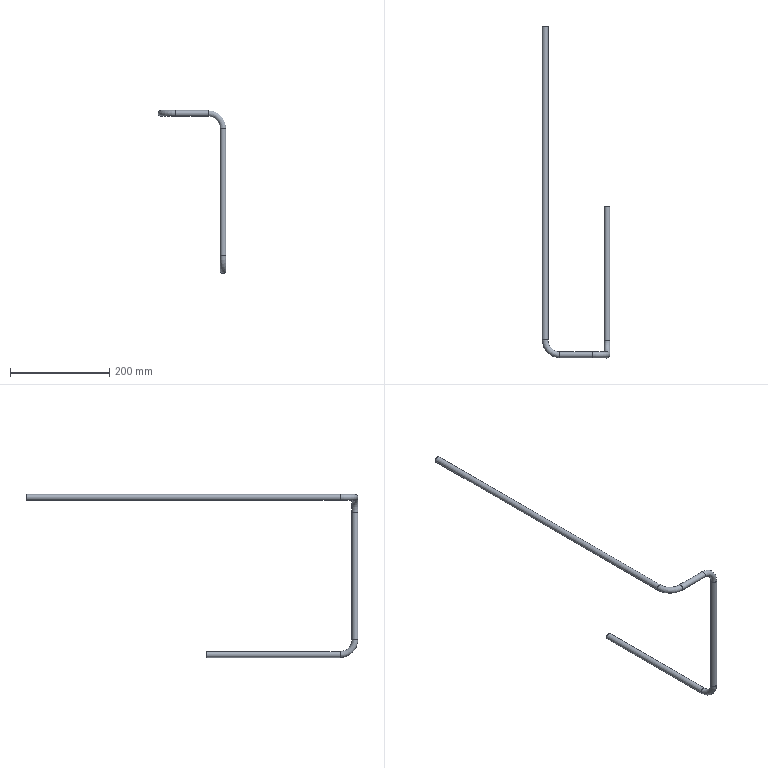Part | NX | features solid 2 | 1 solid | 9 faces | box 137 x 670 x 329.5 mm | volume 154703 mm3 | cylinder 4 | torus 3 | plane 2 | commonest cylinder face diameters 12 x4
STEP:
#1=CARTESIAN_POINT('',(125.,135.,-479.));
#2=VERTEX_POINT('',#1);
#3=CARTESIAN_POINT('',(125.,135.,-485.));
#4=DIRECTION('',(0.,1.,0.));
#5=DIRECTION('',(0.,0.,1.));
#6=AXIS2_PLACEMENT_3D('',#3,#4,#5);
#7=CIRCLE('',#6,6.);
#8=EDGE_CURVE('',#2,#2,#7,.T.);
#9=ORIENTED_EDGE('',*,*,#8,.T.);
#10=EDGE_LOOP('',(#9));
#11=FACE_BOUND('',#10,.T.);
#12=CARTESIAN_POINT('',(125.,405.,-479.));
#13=VERTEX_POINT('',#12);
#14=CARTESIAN_POINT('',(125.,405.,-485.));
#15=DIRECTION('',(0.,1.,0.));
#16=DIRECTION('',(0.,0.,1.));
#17=AXIS2_PLACEMENT_3D('',#14,#15,#16);
#18=CIRCLE('',#17,6.);
#19=EDGE_CURVE('',#13,#13,#18,.T.);
#20=ORIENTED_EDGE('',*,*,#19,.F.);
#21=EDGE_LOOP('',(#20));
#22=FACE_BOUND('',#21,.T.);
#23=CARTESIAN_POINT('',(125.,135.,-485.));
#24=DIRECTION('',(0.,1.,0.));
#25=DIRECTION('',(-1.,0.,0.));
#26=AXIS2_PLACEMENT_3D('',#23,#24,#25);
#27=CYLINDRICAL_SURFACE('',#26,6.);
#28=ADVANCED_FACE('',(#11,#22),#27,.T.);
#29=CARTESIAN_POINT('',(125.,111.,-455.));
#30=VERTEX_POINT('',#29);
#31=CARTESIAN_POINT('',(125.,105.,-455.));
#32=DIRECTION('',(0.,0.,-1.));
#33=DIRECTION('',(0.,1.,0.));
#34=AXIS2_PLACEMENT_3D('',#31,#32,#33);
#35=CIRCLE('',#34,6.);
#36=EDGE_CURVE('',#30,#30,#35,.T.);
#37=ORIENTED_EDGE('',*,*,#36,.T.);
#38=EDGE_LOOP('',(#37));
#39=FACE_BOUND('',#38,.T.);
#40=ORIENTED_EDGE('',*,*,#8,.F.);
#41=EDGE_LOOP('',(#40));
#42=FACE_BOUND('',#41,.T.);
#43=CARTESIAN_POINT('',(125.,135.,-455.));
#44=DIRECTION('',(1.,0.,0.));
#45=DIRECTION('',(0.,0.,-1.));
#46=AXIS2_PLACEMENT_3D('',#43,#44,#45);
#47=TOROIDAL_SURFACE('',#46,30.,6.);
#48=ADVANCED_FACE('',(#39,#42),#47,.T.);
#49=CARTESIAN_POINT('',(125.,111.,-197.5));
#50=VERTEX_POINT('',#49);
#51=CARTESIAN_POINT('',(125.,105.,-197.5));
#52=DIRECTION('',(0.,0.,-1.));
#53=DIRECTION('',(0.,1.,0.));
#54=AXIS2_PLACEMENT_3D('',#51,#52,#53);
#55=CIRCLE('',#54,6.);
#56=EDGE_CURVE('',#50,#50,#55,.T.);
#57=ORIENTED_EDGE('',*,*,#56,.T.);
#58=EDGE_LOOP('',(#57));
#59=FACE_BOUND('',#58,.T.);
#60=ORIENTED_EDGE('',*,*,#36,.F.);
#61=EDGE_LOOP('',(#60));
#62=FACE_BOUND('',#61,.T.);
#63=CARTESIAN_POINT('',(125.,105.,-197.5));
#64=DIRECTION('',(0.,0.,-1.));
#65=DIRECTION('',(-1.,0.,0.));
#66=AXIS2_PLACEMENT_3D('',#63,#64,#65);
#67=CYLINDRICAL_SURFACE('',#66,6.);
#68=ADVANCED_FACE('',(#59,#62),#67,.T.);
#69=CARTESIAN_POINT('',(95.,111.,-167.5));
#70=VERTEX_POINT('',#69);
#71=CARTESIAN_POINT('',(95.,105.,-167.5));
#72=DIRECTION('',(1.,0.,0.));
#73=DIRECTION('',(0.,1.,0.));
#74=AXIS2_PLACEMENT_3D('',#71,#72,#73);
#75=CIRCLE('',#74,6.);
#76=EDGE_CURVE('',#70,#70,#75,.T.);
#77=ORIENTED_EDGE('',*,*,#76,.T.);
#78=EDGE_LOOP('',(#77));
#79=FACE_BOUND('',#78,.T.);
#80=ORIENTED_EDGE('',*,*,#56,.F.);
#81=EDGE_LOOP('',(#80));
#82=FACE_BOUND('',#81,.T.);
#83=CARTESIAN_POINT('',(95.,105.,-197.5));
#84=DIRECTION('',(0.,1.,0.));
#85=DIRECTION('',(0.,0.,1.));
#86=AXIS2_PLACEMENT_3D('',#83,#84,#85);
#87=TOROIDAL_SURFACE('',#86,30.,6.);
#88=ADVANCED_FACE('',(#79,#82),#87,.T.);
#89=CARTESIAN_POINT('',(30.,111.,-167.5));
#90=VERTEX_POINT('',#89);
#91=CARTESIAN_POINT('',(30.,105.,-167.5));
#92=DIRECTION('',(1.,0.,0.));
#93=DIRECTION('',(0.,1.,0.));
#94=AXIS2_PLACEMENT_3D('',#91,#92,#93);
#95=CIRCLE('',#94,6.);
#96=EDGE_CURVE('',#90,#90,#95,.T.);
#97=ORIENTED_EDGE('',*,*,#96,.T.);
#98=EDGE_LOOP('',(#97));
#99=FACE_BOUND('',#98,.T.);
#100=ORIENTED_EDGE('',*,*,#76,.F.);
#101=EDGE_LOOP('',(#100));
#102=FACE_BOUND('',#101,.T.);
#103=CARTESIAN_POINT('',(30.,105.,-167.5));
#104=DIRECTION('',(1.,0.,0.));
#105=DIRECTION('',(0.,0.,-1.));
#106=AXIS2_PLACEMENT_3D('',#103,#104,#105);
#107=CYLINDRICAL_SURFACE('',#106,6.);
#108=ADVANCED_FACE('',(#99,#102),#107,.T.);
#109=CARTESIAN_POINT('',(6.,135.,-167.5));
#110=VERTEX_POINT('',#109);
#111=CARTESIAN_POINT('',(0.,135.,-167.5));
#112=DIRECTION('',(0.,-1.,0.));
#113=DIRECTION('',(1.,0.,0.));
#114=AXIS2_PLACEMENT_3D('',#111,#112,#113);
#115=CIRCLE('',#114,6.);
#116=EDGE_CURVE('',#110,#110,#115,.T.);
#117=ORIENTED_EDGE('',*,*,#116,.T.);
#118=EDGE_LOOP('',(#117));
#119=FACE_BOUND('',#118,.T.);
#120=ORIENTED_EDGE('',*,*,#96,.F.);
#121=EDGE_LOOP('',(#120));
#122=FACE_BOUND('',#121,.T.);
#123=CARTESIAN_POINT('',(30.,135.,-167.5));
#124=DIRECTION('',(0.,0.,1.));
#125=DIRECTION('',(1.,0.,0.));
#126=AXIS2_PLACEMENT_3D('',#123,#124,#125);
#127=TOROIDAL_SURFACE('',#126,30.,6.);
#128=ADVANCED_FACE('',(#119,#122),#127,.T.);
#129=ORIENTED_EDGE('',*,*,#116,.F.);
#130=EDGE_LOOP('',(#129));
#131=FACE_BOUND('',#130,.T.);
#132=CARTESIAN_POINT('',(6.,769.,-167.5));
#133=VERTEX_POINT('',#132);
#134=CARTESIAN_POINT('',(0.,769.,-167.5));
#135=DIRECTION('',(0.,-1.,0.));
#136=DIRECTION('',(1.,0.,0.));
#137=AXIS2_PLACEMENT_3D('',#134,#135,#136);
#138=CIRCLE('',#137,6.);
#139=EDGE_CURVE('',#133,#133,#138,.T.);
#140=ORIENTED_EDGE('',*,*,#139,.T.);
#141=EDGE_LOOP('',(#140));
#142=FACE_BOUND('',#141,.T.);
#143=CARTESIAN_POINT('',(0.,135.,-167.5));
#144=DIRECTION('',(0.,1.,0.));
#145=DIRECTION('',(-1.,0.,0.));
#146=AXIS2_PLACEMENT_3D('',#143,#144,#145);
#147=CYLINDRICAL_SURFACE('',#146,6.);
#148=ADVANCED_FACE('',(#131,#142),#147,.T.);
#149=ORIENTED_EDGE('',*,*,#19,.T.);
#150=EDGE_LOOP('',(#149));
#151=FACE_BOUND('',#150,.T.);
#152=CARTESIAN_POINT('',(125.,405.,-485.));
#153=DIRECTION('',(0.,1.,0.));
#154=DIRECTION('',(0.,0.,1.));
#155=AXIS2_PLACEMENT_3D('',#152,#153,#154);
#156=PLANE('',#155);
#157=ADVANCED_FACE('',(#151),#156,.T.);
#158=ORIENTED_EDGE('',*,*,#139,.F.);
#159=EDGE_LOOP('',(#158));
#160=FACE_BOUND('',#159,.T.);
#161=CARTESIAN_POINT('',(0.,769.,-167.5));
#162=DIRECTION('',(0.,-1.,0.));
#163=DIRECTION('',(1.,0.,0.));
#164=AXIS2_PLACEMENT_3D('',#161,#162,#163);
#165=PLANE('',#164);
#166=ADVANCED_FACE('',(#160),#165,.F.);
#167=CLOSED_SHELL('',(#28,#48,#68,#88,#108,#128,#148,#157,#166));
#168=MANIFOLD_SOLID_BREP('',#167);
#169=(LENGTH_UNIT()NAMED_UNIT(*)SI_UNIT(.MILLI.,.METRE.));
#170=UNCERTAINTY_MEASURE_WITH_UNIT(LENGTH_MEASURE(0.00001),#169,'','');
#171=(NAMED_UNIT(*)PLANE_ANGLE_UNIT()SI_UNIT($,.RADIAN.));
#172=(NAMED_UNIT(*)SI_UNIT($,.STERADIAN.)SOLID_ANGLE_UNIT());
#173=(GEOMETRIC_REPRESENTATION_CONTEXT(3)GLOBAL_UNCERTAINTY_ASSIGNED_CONTEXT((#170))GLOBAL_UNIT_ASSIGNED_CONTEXT((#169,#171,#172))REPRESENTATION_CONTEXT('',''));
#174=ADVANCED_BREP_SHAPE_REPRESENTATION('',(#168),#173);